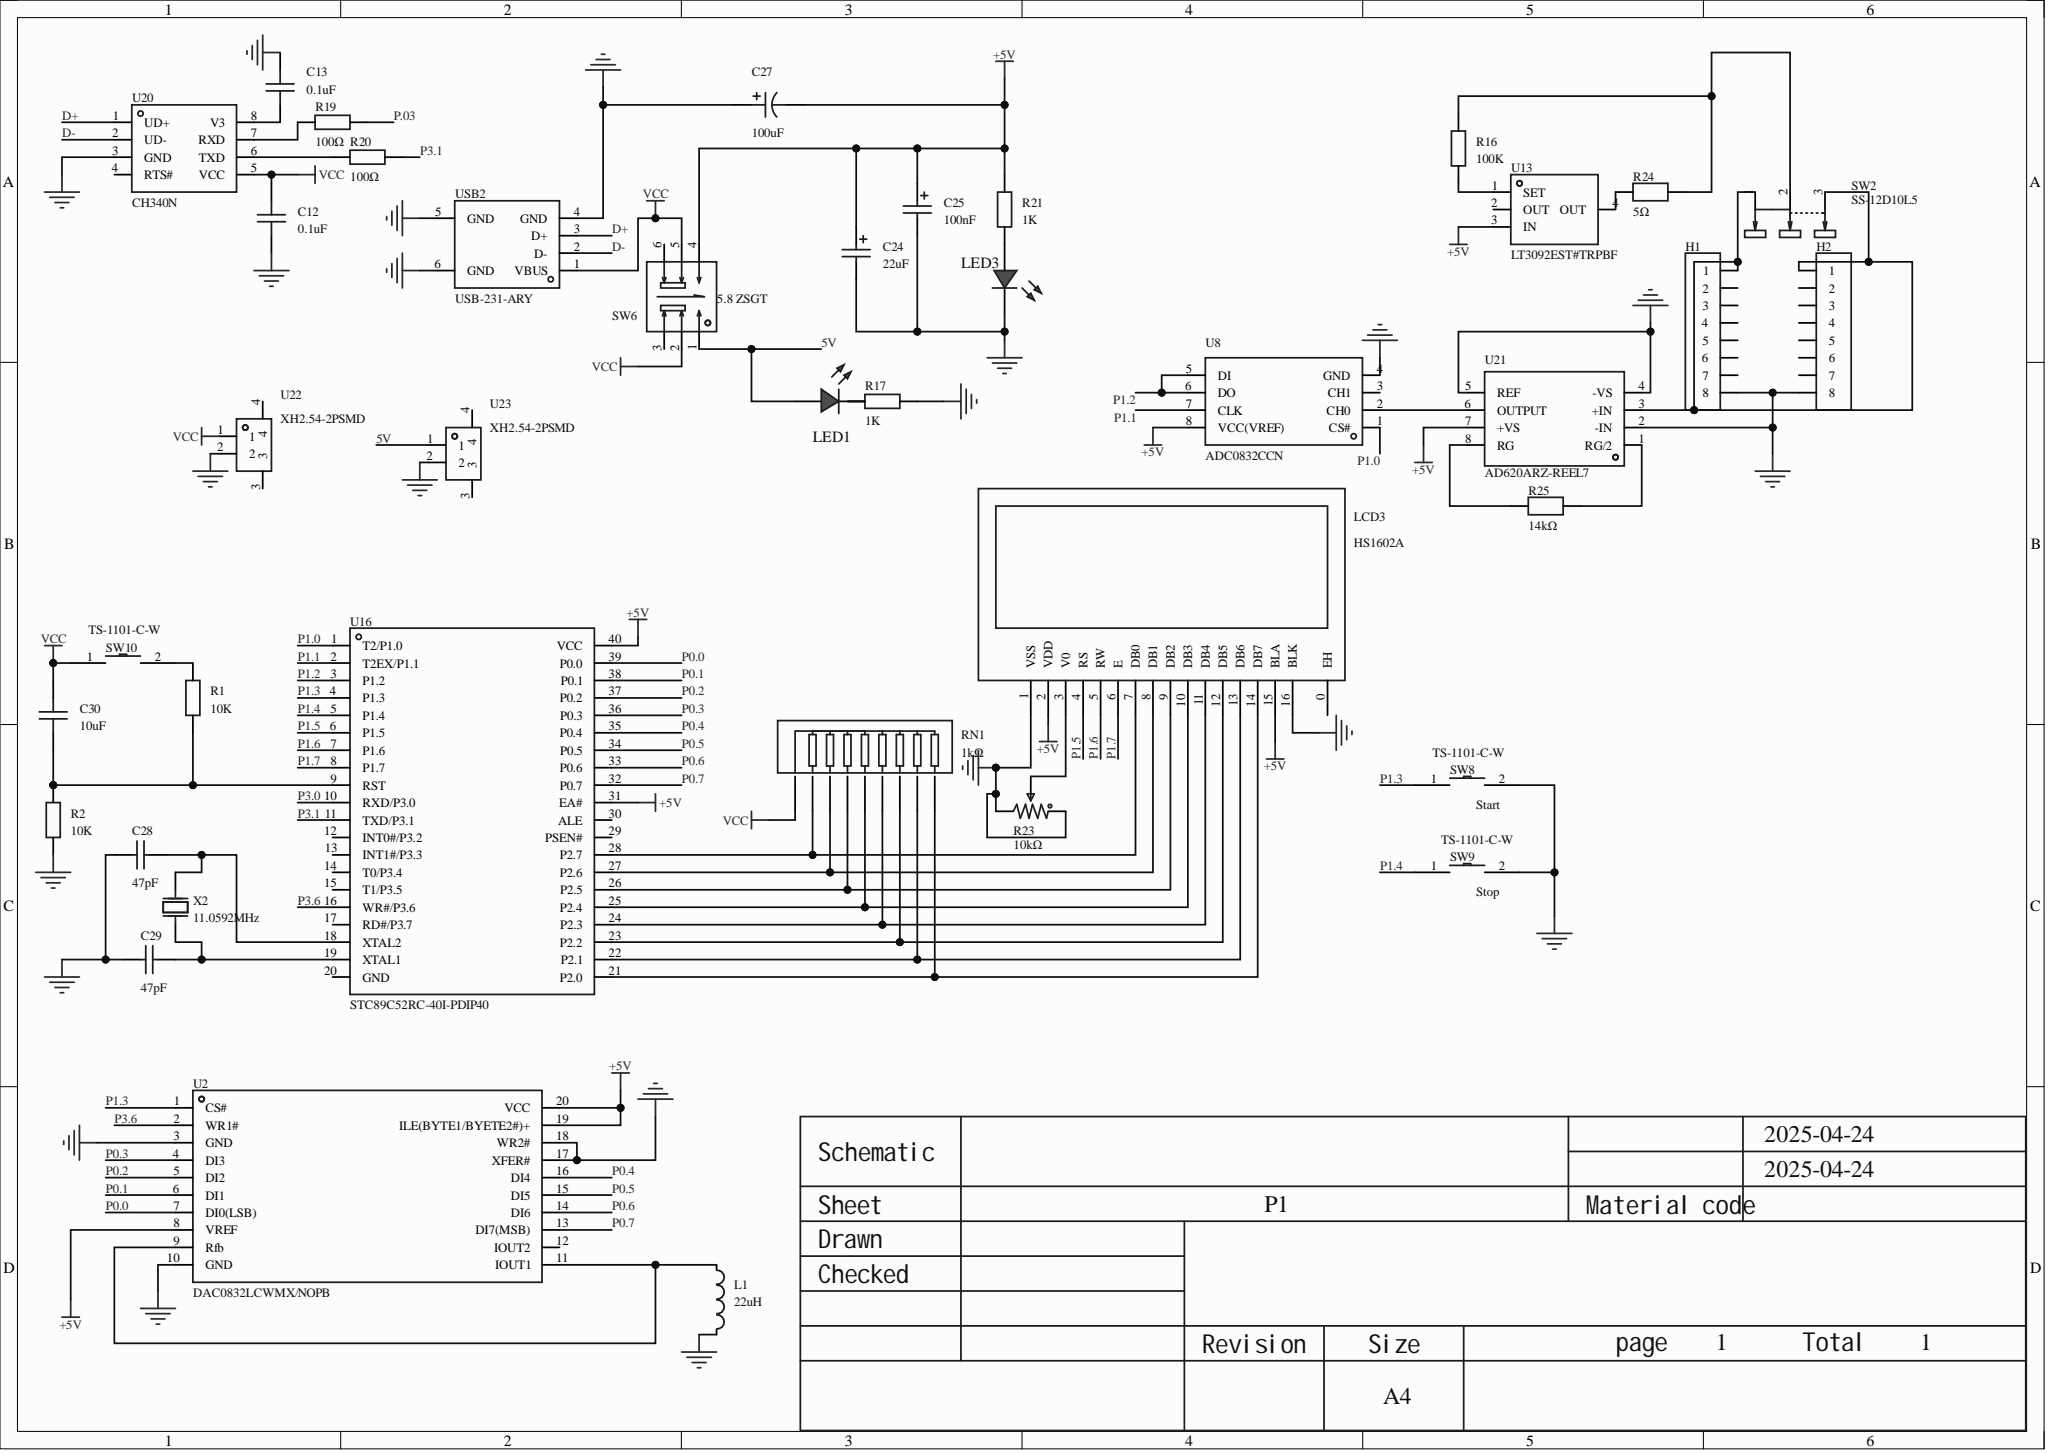Circuit board | Altium Designer | 40 parts | 50 nets
Bill of materials:
Comment,Description,Designator,Footprint,LibRef,Quantity
"0.1uF","","C12, C13","C0603","CAP_0603","2"
"22uF","Capacitance: 220uF; tolerance: ±20%; rated voltage: 6.3V; equivalent series resistance (ESR): 35mΩ@100kHz;","C24","CAP-SMD_L3.5-W2.8-R-RD","6TPE220MAZB","1"
"100nF","Capacitance: 100nF; tolerance: ±10%; rated voltage: 35V; equivalent series resistance: 24Ω@100kHz;","C25","CASE-A_3216","TAJA104K035RNJ","1"
"100uF","Capacitance: 100uF; tolerance: ±20%; rated voltage: 50V; ripple current: 300mA@100kHz; equivalent series resistance: 600mΩ@100kHz;","C27","CAP-SMD_BD8.1-L8.3-W8.3-LS9.3-FD","GVE1H107M0810CNVC","1"
"47pF","Capacitance: 47pF; tolerance: ±5%; rated voltage: 50V; dielectric (temperature coefficient): C0G;","C28, C29","C0603","CL10C470JB8NNNC","2"
"10uF","Capacitance: 10uF; tolerance: ±10%; rated voltage: 10V; temperature coefficient: X5R;","C30","C0603","CGA0603X5R106K100JT","1"
"","","H1, H2","HDR-TH_8P-P2.54-V-F-1","HDR-F_2.54_1x8P","2"
"22uH","Inductance: 22uH; tolerance: ±20%; rated current: 8A; saturation current (Isat): -; type: toroidal inductor; Q factor: -;","L1","IND-TH_BD14.7-2P-P4.00","PDMTAT044125-220MWU","1"
"HS1602A","Controller chip: SPLC780; size (inch): 2;","LCD3","LCD1602","HS1602A","1"
"","","LED1, LED3","LED_0603","LED_0603-R","2"
"10K","","R1, R2","R0603","Res_0603","2"
"100K","","R16","R0603","Res_0603","1"
"1K","","R17, R21","R0603","Res_0603","2"
"100Ω","","R19, R20","R0603","Res_0603","2"
"10kΩ","Resistance: 10kΩ; tolerance: ±25%; power: 150mW; temperature coefficient: ±250ppm/?;","R23","RES-ADJ-SMD_3P-L3.0-W3.8-P1.75-BR","TC33X-2-103E","1"
"5Ω","Resistor type: ceramic resistor; resistance: 5Ω; tolerance: ±0.1%; power: 1W; temperature coefficient: ±25ppm/?;","R24","R2512","HoAR2512-1W-5R-0.1%-TCR25","1"
"14kΩ","Resistor type: thick-film resistor; resistance: 14kΩ; tolerance: ±1%; power: 100mW; operating voltage: 75V; temperature coefficient: ±100ppm/?;","R25","R0603","FRC0603F1402TS","1"
"1kΩ","Number of resistors: 8; resistance: 1kΩ; tolerance: ±5%; power per element: 125mW; temperature coefficient: ±100ppm/?;","RN1","RES-ARRAY-TH_9P-P2.54-D1.0","A09-102JP","1"
"SS-12D10L5","Circuit structure: SPDT; mounting: through-hole; switch colour: black; rated current (DC): 3A; rated voltage (DC): 125V; rated current (AC): 3A; rated voltage (AC): 125V; mechanical life: 1 ten-thousand cycles;","SW2","SW-TH_SS-12D10L5","SS-12D10L5","1"
"5.8 ZSGT","Circuit structure: DPDT; self-lock / no-lock: self-lock; mounting: through-hole; contact current: 110mA; rated voltage (DC): 30V; with lamp: without; actuating force: 1.5N; mechanical life: 10 ten-thousand cycles;","SW6","SW-TH_5.8ZSGT","5.8 ZSGT","1"
"TS-1101-C-W","Circuit structure: SPST; button shape: rectangular button; actuating force: 260gf; mounting: surface mount; switch length: 6mm; switch width: 3.6mm; switch height: 2.5mm; with bracket: without; contact current: 50mA; rated voltage (AC): -; rated voltage (DC): 12V; rated power: -; insulation resistance: -; with lamp: none; mechanical life: 5 ten-thousand cycles;","SW8, SW9, SW10","SW-SMD_L6.0-W3.3-LS8.0","TS-1101-C-W","3"
"DAC0832LCWMX/NOPB","","U2","SOIC-20_L13.0-W7.6-P1.27-LS10.3-BL","DAC0832LCWMX/NOPB","1"
"ADC0832CCN","8BIT serial A/D converter chip","U8","DIP-8_L9.7-W6.4-P2.54-LS7.6-BL","ADC0832CCN_C5357","1"
"LT3092EST#TRPBF","Operating voltage: 1.2V~40V; output current: 200mA;","U13","SOT-223-4_L6.5-W3.5-P2.30-LS7.0-BR","LT3092EST#TRPBF","1"
"STC89C52RC-40I-PDIP40","CPU core: 51 series; application field: -;","U16","DIP-40_L52.0-W13.7-P2.54-LS15.2-BL","STC89C52RC-40I-PDIP40","1"
"CH340N","Application function: USB to serial; interface protocol: USB 2.0; channels: 1; data rate: 2Mbps;","U20","SOP-8_L4.9-W3.9-P1.27-LS6.0-BL","CH340N","1"
"AD620ARZ-REEL7","Number of amplifiers: single; input bias current (Ib): 500pA; input offset voltage (Vos): 30uV; gain-bandwidth product (GBP): -; slew rate (SR): 1.2V/us; bandwidth (-3db): 1MHz;","U21","SOIC-8_L5.0-W4.0-P1.27-LS6.0-BL","AD620ARZ-REEL7","1"
"XH2.54-2PSMD","","U22, U23","CONN-SMD_XH2.54-2PSMD","XH2.54-2PSMD","2"
"USB-231-ARY","Connector type: Type-A; standard: USB 2.0; gender: female; number of ports: 1; number of contacts: 4P; mounting: right-angle through-hole; rated current - power: 1.5A; contact material: -; contact plating: -; operating temperature range: -20℃~+70℃; soldering temperature (max): 260℃;","USB2","USB-A-TH_USB-231-ARY","USB-231-ARY","1"
"11.059MHz","Crystal type: through-hole crystal; frequency: 11.059MHz; room-temperature tolerance: ±20ppm; load capacitance: 20pF; frequency stability: ±30ppm;","X2","HC-49US_L11.5-W4.5-P4.88","X49SD110592MSD2SC","1"
Netlist (Protel format):
[
C12
C0603
0.1uF



]
[
C13
C0603
0.1uF



]
[
C24
CAP-SMD_L3.5-W2.8-R-RD
22uF



]
[
C25
CASE-A_3216
100nF



]
[
C27
CAP-SMD_BD8.1-L8.3-W8.3-LS9.3-FD
100uF



]
[
C28
C0603
47pF



]
[
C29
C0603
47pF



]
[
C30
C0603
10uF



]
[
H1
HDR-TH_8P-P2.54-V-F-1




]
[
H2
HDR-TH_8P-P2.54-V-F-1




]
[
L1
IND-TH_BD14.7-2P-P4.00
22uH



]
[
LCD3
LCD1602
HS1602A



]
[
LED1
LED_0603




]
[
LED3
LED_0603




]
[
R1
R0603
10K



]
[
R2
R0603
10K



]
[
R16
R0603
100K



]
[
R17
R0603
1K



]
[
R19
R0603
100Ω



]
[
R20
R0603
100Ω



]
[
R21
R0603
1K



]
[
R23
RES-ADJ-SMD_3P-L3.0-W3.8-P1.75-BR
10kΩ



]
[
R24
R2512
5Ω



]
[
R25
R0603
14kΩ



]
[
RN1
RES-ARRAY-TH_9P-P2.54-D1.0
1kΩ



]
[
SW2
SW-TH_SS-12D10L5
SS-12D10L5



]
[
SW6
SW-TH_5.8ZSGT
5.8 ZSGT



]
[
SW8
SW-SMD_L6.0-W3.3-LS8.0
TS-1101-C-W



]
[
SW9
SW-SMD_L6.0-W3.3-LS8.0
TS-1101-C-W



]
[
SW10
SW-SMD_L6.0-W3.3-LS8.0
TS-1101-C-W



]
[
U2
SOIC-20_L13.0-W7.6-P1.27-LS10.3-BL
DAC0832LCWMX/NOPB



]
[
U8
DIP-8_L9.7-W6.4-P2.54-LS7.6-BL
ADC0832CCN



]
[
U13
SOT-223-4_L6.5-W3.5-P2.30-LS7.0-BR
LT3092EST#TRPBF



]
[
U16
DIP-40_L52.0-W13.7-P2.54-LS15.2-BL
STC89C52RC-40I-PDIP40



]
[
U20
SOP-8_L4.9-W3.9-P1.27-LS6.0-BL
CH340N



]
[
U21
SOIC-8_L5.0-W4.0-P1.27-LS6.0-BL
AD620ARZ-REEL7



]
[
U22
CONN-SMD_XH2.54-2PSMD
XH2.54-2PSMD



]
[
U23
CONN-SMD_XH2.54-2PSMD
XH2.54-2PSMD



]
[
USB2
USB-A-TH_USB-231-ARY
USB-231-ARY



]
[
X2
HC-49US_L11.5-W4.5-P4.88
11.0592MHz



]
(
VCC
C12-2
C30-2
RN1-1
SW6-2
SW6-5
SW10-1
U20-5
U22-1
USB2-1
)
(
P3.6
U2-2
U16-16
)
(
P3.1
R20-2
U16-11
)
(
P1.7
LCD3-6
U16-8
)
(
P1.6
LCD3-5
U16-7
)
(
P1.5
LCD3-4
U16-6
)
(
P1.4
SW9-1
U16-5
)
(
P1.3
SW8-1
U2-1
U16-4
)
(
P1.2
U8-5
U8-6
U16-3
)
(
P1.1
U8-7
U16-2
)
(
P1.0
U8-1
U16-1
)
(
P0.7
U2-13
U16-32
)
(
P0.6
U2-14
U16-33
)
(
P0.5
U2-15
U16-34
)
(
P0.4
U2-16
U16-35
)
(
P0.3
U2-4
U16-36
)
(
P0.2
U2-5
U16-37
)
(
P0.1
U2-6
U16-38
)
(
P0.0
U2-7
U16-39
)
(
NetU8_2
U8-2
U21-6
)
(
NetR25_2
R25-2
U21-1
)
(
NetR25_1
R25-1
U21-8
)
(
NetR24_1
R24-1
U13-4
)
(
NetR20_1
R20-1
U20-6
)
(
NetR19_1
R19-1
U20-7
)
(
NetR16_2
R16-2
R24-2
SW2-2
)
(
NetR16_1
R16-1
U13-1
)
(
NetR1_2
R1-2
SW10-2
)
(
NetLED3_2
LED3-2
R21-1
)
(
NetLED1_1
LED1-1
R17-1
)
(
NetLCD3_14
LCD3-14
RN1-9
U16-21
)
(
NetLCD3_13
LCD3-13
RN1-8
U16-22
)
(
NetLCD3_12
LCD3-12
RN1-7
U16-23
)
(
NetLCD3_11
LCD3-11
RN1-6
U16-24
)
(
NetLCD3_10
LCD3-10
RN1-5
U16-25
)
(
NetLCD3_9
LCD3-9
RN1-4
U16-26
)
(
NetLCD3_8
LCD3-8
RN1-3
U16-27
)
(
NetLCD3_7
LCD3-7
RN1-2
U16-28
)
(
NetLCD3_3
LCD3-3
R23-2
)
(
NetL1_1
L1-1
U2-9
U2-11
)
(
NetH1_1
H1-1
H2-1
SW2-1
SW2-3
U21-3
)
(
NetC30_1
C30-1
R1-1
R2-2
U16-9
)
(
NetC29_2
C29-2
U16-19
X2-2
)
(
NetC28_2
C28-2
U16-18
X2-1
)
(
NetC13_2
C13-2
U20-8
)
(
GND
C12-1
C13-1
C24-2
C25-2
C27-1
C28-1
C29-1
H1-8
H2-8
L1-2
LCD3-1
LCD3-16
LED3-1
R2-1
R17-2
R23-1
R23-3
SW8-2
SW9-2
U2-3
U2-10
U2-17
U2-18
U8-4
U20-3
U21-2
U21-4
U21-5
U22-2
U23-2
USB2-4
USB2-5
USB2-6
)
(
D-
U20-2
USB2-2
)
(
D+
U20-1
USB2-3
)
(
+5V
C24-1
C25-1
C27-2
LCD3-2
LCD3-15
R21-2
SW6-4
U2-8
U2-19
U2-20
U8-8
U13-3
U16-31
U16-40
U21-7
)
(
5V
LED1-2
SW6-1
U23-1
)